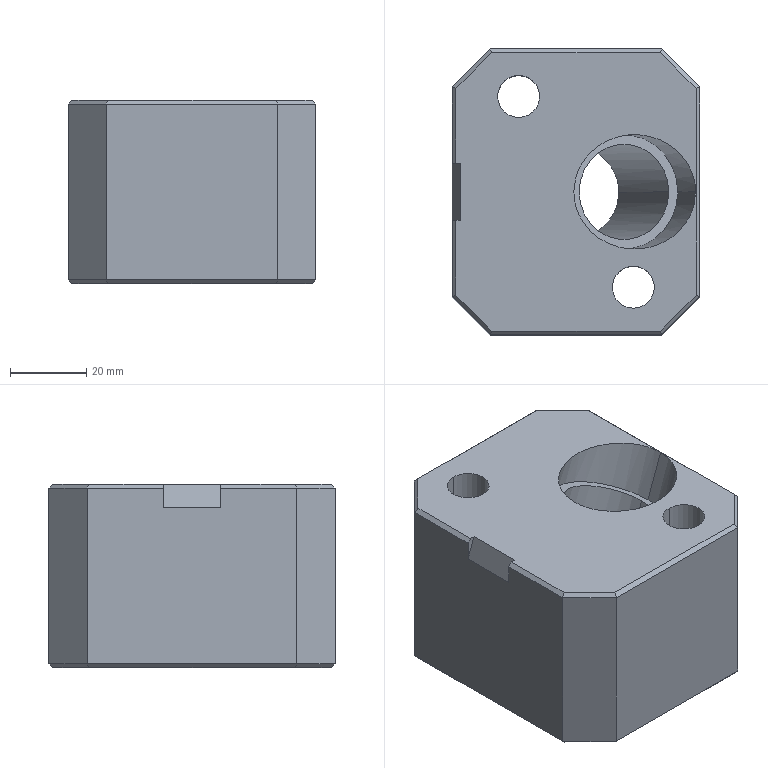Part | Creo | 3 solids | 49 faces | box 65 x 75 x 48 mm | volume 184573 mm3 | plane 33 | cylinder 16 | commonest cylinder face diameters 11 x4 18 x4 11.98 x2 12 x2 25 x2 30 x2
STEP:
#1=CARTESIAN_POINT('',(-250.936,145.997,1.));
#2=VERTEX_POINT('',#1);
#3=CARTESIAN_POINT('',(-250.936,163.997,1.));
#4=VERTEX_POINT('',#3);
#5=CARTESIAN_POINT('',(-250.936,154.997,1.));
#6=DIRECTION('',(0.,0.,-1.));
#7=DIRECTION('',(0.,-1.,0.));
#8=AXIS2_PLACEMENT_3D('',#5,#6,#7);
#9=CIRCLE('',#8,9.);
#10=EDGE_CURVE('',#2,#4,#9,.T.);
#11=ORIENTED_EDGE('',*,*,#10,.F.);
#12=CARTESIAN_POINT('',(-250.936,154.997,1.));
#13=DIRECTION('',(0.,0.,-1.));
#14=DIRECTION('',(0.,1.,0.));
#15=AXIS2_PLACEMENT_3D('',#12,#13,#14);
#16=CIRCLE('',#15,9.);
#17=EDGE_CURVE('',#4,#2,#16,.T.);
#18=ORIENTED_EDGE('',*,*,#17,.F.);
#19=EDGE_LOOP('',(#11,#18));
#20=FACE_OUTER_BOUND('',#19,.F.);
#21=CARTESIAN_POINT('',(-250.936,149.497,1.));
#22=VERTEX_POINT('',#21);
#23=CARTESIAN_POINT('',(-250.936,160.497,1.));
#24=VERTEX_POINT('',#23);
#25=CARTESIAN_POINT('',(-250.936,154.997,1.));
#26=DIRECTION('',(0.,0.,1.));
#27=DIRECTION('',(0.,-1.,0.));
#28=AXIS2_PLACEMENT_3D('',#25,#26,#27);
#29=CIRCLE('',#28,5.5);
#30=EDGE_CURVE('',#22,#24,#29,.T.);
#31=ORIENTED_EDGE('',*,*,#30,.F.);
#32=CARTESIAN_POINT('',(-250.936,154.997,1.));
#33=DIRECTION('',(0.,0.,1.));
#34=DIRECTION('',(0.,1.,0.));
#35=AXIS2_PLACEMENT_3D('',#32,#33,#34);
#36=CIRCLE('',#35,5.5);
#37=EDGE_CURVE('',#24,#22,#36,.T.);
#38=ORIENTED_EDGE('',*,*,#37,.F.);
#39=EDGE_LOOP('',(#31,#38));
#40=FACE_BOUND('',#39,.F.);
#41=CARTESIAN_POINT('',(-250.936,154.997,1.));
#42=DIRECTION('',(0.,0.,1.));
#43=DIRECTION('',(0.,-1.,0.));
#44=AXIS2_PLACEMENT_3D('',#41,#42,#43);
#45=PLANE('',#44);
#46=ADVANCED_FACE('',(#20,#40),#45,.F.);
#47=ORIENTED_EDGE('',*,*,#10,.T.);
#48=CARTESIAN_POINT('',(-250.936,163.997,-10.));
#49=VERTEX_POINT('',#48);
#50=CARTESIAN_POINT('',(-250.936,163.997,-10.));
#51=DIRECTION('',(0.,0.,1.));
#52=VECTOR('',#51,11.);
#53=LINE('',#50,#52);
#54=EDGE_CURVE('',#49,#4,#53,.T.);
#55=ORIENTED_EDGE('',*,*,#54,.F.);
#56=CARTESIAN_POINT('',(-250.936,145.997,-10.));
#57=VERTEX_POINT('',#56);
#58=CARTESIAN_POINT('',(-250.936,154.997,-10.));
#59=DIRECTION('',(0.,0.,1.));
#60=DIRECTION('',(0.,1.,0.));
#61=AXIS2_PLACEMENT_3D('',#58,#59,#60);
#62=CIRCLE('',#61,9.);
#63=EDGE_CURVE('',#49,#57,#62,.T.);
#64=ORIENTED_EDGE('',*,*,#63,.T.);
#65=CARTESIAN_POINT('',(-250.936,145.997,-10.));
#66=DIRECTION('',(0.,0.,1.));
#67=VECTOR('',#66,11.);
#68=LINE('',#65,#67);
#69=EDGE_CURVE('',#57,#2,#68,.T.);
#70=ORIENTED_EDGE('',*,*,#69,.T.);
#71=EDGE_LOOP('',(#47,#55,#64,#70));
#72=FACE_OUTER_BOUND('',#71,.F.);
#73=CARTESIAN_POINT('',(-250.936,154.997,-10.));
#74=DIRECTION('',(0.,0.,1.));
#75=DIRECTION('',(0.,-1.,0.));
#76=AXIS2_PLACEMENT_3D('',#73,#74,#75);
#77=CYLINDRICAL_SURFACE('',#76,9.);
#78=ADVANCED_FACE('',(#72),#77,.F.);
#79=ORIENTED_EDGE('',*,*,#17,.T.);
#80=ORIENTED_EDGE('',*,*,#69,.F.);
#81=CARTESIAN_POINT('',(-250.936,154.997,-10.));
#82=DIRECTION('',(0.,0.,1.));
#83=DIRECTION('',(0.,-1.,0.));
#84=AXIS2_PLACEMENT_3D('',#81,#82,#83);
#85=CIRCLE('',#84,9.);
#86=EDGE_CURVE('',#57,#49,#85,.T.);
#87=ORIENTED_EDGE('',*,*,#86,.T.);
#88=ORIENTED_EDGE('',*,*,#54,.T.);
#89=EDGE_LOOP('',(#79,#80,#87,#88));
#90=FACE_OUTER_BOUND('',#89,.F.);
#91=CARTESIAN_POINT('',(-250.936,154.997,-10.));
#92=DIRECTION('',(0.,0.,1.));
#93=DIRECTION('',(0.,-1.,0.));
#94=AXIS2_PLACEMENT_3D('',#91,#92,#93);
#95=CYLINDRICAL_SURFACE('',#94,9.);
#96=ADVANCED_FACE('',(#90),#95,.F.);
#97=CARTESIAN_POINT('',(-213.85,166.497,-10.));
#98=VERTEX_POINT('',#97);
#99=CARTESIAN_POINT('',(-204.436,157.083,-10.));
#100=VERTEX_POINT('',#99);
#101=CARTESIAN_POINT('',(-213.85,166.497,-10.));
#102=DIRECTION('',(0.7071,-0.7071,0.));
#103=VECTOR('',#102,13.314);
#104=LINE('',#101,#103);
#105=EDGE_CURVE('',#98,#100,#104,.T.);
#106=ORIENTED_EDGE('',*,*,#105,.F.);
#107=CARTESIAN_POINT('',(-258.022,166.497,-10.));
#108=VERTEX_POINT('',#107);
#109=CARTESIAN_POINT('',(-213.85,166.497,-10.));
#110=DIRECTION('',(-1.,0.,0.));
#111=VECTOR('',#110,44.172);
#112=LINE('',#109,#111);
#113=EDGE_CURVE('',#98,#108,#112,.T.);
#114=ORIENTED_EDGE('',*,*,#113,.T.);
#115=CARTESIAN_POINT('',(-267.436,157.083,-10.));
#116=VERTEX_POINT('',#115);
#117=CARTESIAN_POINT('',(-267.436,157.083,-10.));
#118=DIRECTION('',(0.7071,0.7071,0.));
#119=VECTOR('',#118,13.314);
#120=LINE('',#117,#119);
#121=EDGE_CURVE('',#116,#108,#120,.T.);
#122=ORIENTED_EDGE('',*,*,#121,.F.);
#123=CARTESIAN_POINT('',(-267.436,102.911,-10.));
#124=VERTEX_POINT('',#123);
#125=CARTESIAN_POINT('',(-267.436,157.083,-10.));
#126=DIRECTION('',(0.,-1.,0.));
#127=VECTOR('',#126,54.172);
#128=LINE('',#125,#127);
#129=EDGE_CURVE('',#116,#124,#128,.T.);
#130=ORIENTED_EDGE('',*,*,#129,.T.);
#131=CARTESIAN_POINT('',(-258.022,93.497,-10.));
#132=VERTEX_POINT('',#131);
#133=CARTESIAN_POINT('',(-258.022,93.497,-10.));
#134=DIRECTION('',(-0.7071,0.7071,0.));
#135=VECTOR('',#134,13.314);
#136=LINE('',#133,#135);
#137=EDGE_CURVE('',#132,#124,#136,.T.);
#138=ORIENTED_EDGE('',*,*,#137,.F.);
#139=CARTESIAN_POINT('',(-213.85,93.497,-10.));
#140=VERTEX_POINT('',#139);
#141=CARTESIAN_POINT('',(-258.022,93.497,-10.));
#142=DIRECTION('',(1.,0.,0.));
#143=VECTOR('',#142,44.172);
#144=LINE('',#141,#143);
#145=EDGE_CURVE('',#132,#140,#144,.T.);
#146=ORIENTED_EDGE('',*,*,#145,.T.);
#147=CARTESIAN_POINT('',(-204.436,102.911,-10.));
#148=VERTEX_POINT('',#147);
#149=CARTESIAN_POINT('',(-204.436,102.911,-10.));
#150=DIRECTION('',(-0.7071,-0.7071,0.));
#151=VECTOR('',#150,13.314);
#152=LINE('',#149,#151);
#153=EDGE_CURVE('',#148,#140,#152,.T.);
#154=ORIENTED_EDGE('',*,*,#153,.F.);
#155=CARTESIAN_POINT('',(-204.436,102.911,-10.));
#156=DIRECTION('',(0.,1.,0.));
#157=VECTOR('',#156,54.172);
#158=LINE('',#155,#157);
#159=EDGE_CURVE('',#148,#100,#158,.T.);
#160=ORIENTED_EDGE('',*,*,#159,.T.);
#161=EDGE_LOOP('',(#106,#114,#122,#130,#138,#146,#154,#160));
#162=FACE_OUTER_BOUND('',#161,.F.);
#163=CARTESIAN_POINT('',(-224.707,129.995,-10.));
#164=VERTEX_POINT('',#163);
#165=CARTESIAN_POINT('',(-251.311,129.995,-10.));
#166=VERTEX_POINT('',#165);
#167=CARTESIAN_POINT('',(-224.707,129.995,-10.));
#168=CARTESIAN_POINT('',(-224.707,128.522,-10.));
#169=CARTESIAN_POINT('',(-225.275,125.338,-10.));
#170=CARTESIAN_POINT('',(-227.815,121.638,-10.));
#171=CARTESIAN_POINT('',(-230.687,119.454,-10.));
#172=CARTESIAN_POINT('',(-233.098,118.289,-10.));
#173=CARTESIAN_POINT('',(-235.181,117.737,-10.));
#174=CARTESIAN_POINT('',(-236.821,117.528,-10.));
#175=CARTESIAN_POINT('',(-238.009,117.479,-10.));
#176=CARTESIAN_POINT('',(-239.198,117.528,-10.));
#177=CARTESIAN_POINT('',(-240.838,117.737,-10.));
#178=CARTESIAN_POINT('',(-242.921,118.289,-10.));
#179=CARTESIAN_POINT('',(-245.331,119.454,-10.));
#180=CARTESIAN_POINT('',(-248.203,121.638,-10.));
#181=CARTESIAN_POINT('',(-250.743,125.338,-10.));
#182=CARTESIAN_POINT('',(-251.311,128.522,-10.));
#183=CARTESIAN_POINT('',(-251.311,129.995,-10.));
#184=B_SPLINE_CURVE_WITH_KNOTS('',3,(#167,#168,#169,#170,#171,#172,#173,#174,#175,#176,#177,#178,#179,#180,#181,#182,#183),.UNSPECIFIED.,.F.,.F.,(4,1,1,1,1,1,1,1,1,1,1,1,1,1,4),(0.,0.125,0.25,0.3125,0.375,0.4375,0.4688,0.5,0.5312,0.5625,0.625,0.6875,0.75,0.875,1.),.UNSPECIFIED.);
#185=EDGE_CURVE('',#164,#166,#184,.T.);
#186=ORIENTED_EDGE('',*,*,#185,.T.);
#187=CARTESIAN_POINT('',(-251.311,129.995,-10.));
#188=CARTESIAN_POINT('',(-251.311,131.468,-10.));
#189=CARTESIAN_POINT('',(-250.743,134.652,-10.));
#190=CARTESIAN_POINT('',(-248.203,138.353,-10.));
#191=CARTESIAN_POINT('',(-245.331,140.537,-10.));
#192=CARTESIAN_POINT('',(-242.921,141.701,-10.));
#193=CARTESIAN_POINT('',(-240.838,142.254,-10.));
#194=CARTESIAN_POINT('',(-239.198,142.463,-10.));
#195=CARTESIAN_POINT('',(-238.009,142.512,-10.));
#196=CARTESIAN_POINT('',(-236.821,142.463,-10.));
#197=CARTESIAN_POINT('',(-235.181,142.254,-10.));
#198=CARTESIAN_POINT('',(-233.098,141.701,-10.));
#199=CARTESIAN_POINT('',(-230.687,140.537,-10.));
#200=CARTESIAN_POINT('',(-227.815,138.353,-10.));
#201=CARTESIAN_POINT('',(-225.275,134.652,-10.));
#202=CARTESIAN_POINT('',(-224.707,131.468,-10.));
#203=CARTESIAN_POINT('',(-224.707,129.995,-10.));
#204=B_SPLINE_CURVE_WITH_KNOTS('',3,(#187,#188,#189,#190,#191,#192,#193,#194,#195,#196,#197,#198,#199,#200,#201,#202,#203),.UNSPECIFIED.,.F.,.F.,(4,1,1,1,1,1,1,1,1,1,1,1,1,1,4),(0.,0.125,0.25,0.3125,0.375,0.4375,0.4688,0.5,0.5312,0.5625,0.625,0.6875,0.75,0.875,1.),.UNSPECIFIED.);
#205=EDGE_CURVE('',#166,#164,#204,.T.);
#206=ORIENTED_EDGE('',*,*,#205,.T.);
#207=EDGE_LOOP('',(#186,#206));
#208=FACE_BOUND('',#207,.F.);
#209=ORIENTED_EDGE('',*,*,#86,.F.);
#210=ORIENTED_EDGE('',*,*,#63,.F.);
#211=EDGE_LOOP('',(#209,#210));
#212=FACE_BOUND('',#211,.F.);
#213=CARTESIAN_POINT('',(-220.936,95.997,-10.));
#214=VERTEX_POINT('',#213);
#215=CARTESIAN_POINT('',(-220.936,113.997,-10.));
#216=VERTEX_POINT('',#215);
#217=CARTESIAN_POINT('',(-220.936,104.997,-10.));
#218=DIRECTION('',(0.,0.,1.));
#219=DIRECTION('',(0.,-1.,0.));
#220=AXIS2_PLACEMENT_3D('',#217,#218,#219);
#221=CIRCLE('',#220,9.);
#222=EDGE_CURVE('',#214,#216,#221,.T.);
#223=ORIENTED_EDGE('',*,*,#222,.F.);
#224=CARTESIAN_POINT('',(-220.936,104.997,-10.));
#225=DIRECTION('',(0.,0.,1.));
#226=DIRECTION('',(0.,1.,0.));
#227=AXIS2_PLACEMENT_3D('',#224,#225,#226);
#228=CIRCLE('',#227,9.);
#229=EDGE_CURVE('',#216,#214,#228,.T.);
#230=ORIENTED_EDGE('',*,*,#229,.F.);
#231=EDGE_LOOP('',(#223,#230));
#232=FACE_BOUND('',#231,.F.);
#233=CARTESIAN_POINT('',(605.564,160.997,-10.));
#234=DIRECTION('',(0.,0.,1.));
#235=DIRECTION('',(-1.,0.,0.));
#236=AXIS2_PLACEMENT_3D('',#233,#234,#235);
#237=PLANE('',#236);
#238=ADVANCED_FACE('',(#162,#208,#212,#232),#237,.F.);
#239=CARTESIAN_POINT('',(-211.613,129.995,25.977));
#240=VERTEX_POINT('',#239);
#241=CARTESIAN_POINT('',(-235.105,129.995,34.527));
#242=VERTEX_POINT('',#241);
#243=CARTESIAN_POINT('',(-223.359,129.995,30.252));
#244=DIRECTION('',(-0.342,0.,-0.9397));
#245=DIRECTION('',(0.9397,0.,-0.342));
#246=AXIS2_PLACEMENT_3D('',#243,#244,#245);
#247=CIRCLE('',#246,12.5);
#248=EDGE_CURVE('',#240,#242,#247,.T.);
#249=ORIENTED_EDGE('',*,*,#248,.T.);
#250=CARTESIAN_POINT('',(-235.105,129.995,34.527));
#251=DIRECTION('',(-0.342,0.,-0.9397));
#252=VECTOR('',#251,47.385);
#253=LINE('',#250,#252);
#254=EDGE_CURVE('',#242,#166,#253,.T.);
#255=ORIENTED_EDGE('',*,*,#254,.T.);
#256=ORIENTED_EDGE('',*,*,#185,.F.);
#257=CARTESIAN_POINT('',(-211.613,129.995,25.977));
#258=DIRECTION('',(-0.342,0.,-0.9397));
#259=VECTOR('',#258,38.286);
#260=LINE('',#257,#259);
#261=EDGE_CURVE('',#240,#164,#260,.T.);
#262=ORIENTED_EDGE('',*,*,#261,.F.);
#263=EDGE_LOOP('',(#249,#255,#256,#262));
#264=FACE_OUTER_BOUND('',#263,.F.);
#265=CARTESIAN_POINT('',(-211.802,129.995,62.004));
#266=DIRECTION('',(-0.342,0.,-0.9397));
#267=DIRECTION('',(-0.9397,0.,0.342));
#268=AXIS2_PLACEMENT_3D('',#265,#266,#267);
#269=CYLINDRICAL_SURFACE('',#268,12.5);
#270=ADVANCED_FACE('',(#264),#269,.F.);
#271=CARTESIAN_POINT('',(-209.263,129.995,25.122));
#272=VERTEX_POINT('',#271);
#273=CARTESIAN_POINT('',(-237.454,129.995,35.382));
#274=VERTEX_POINT('',#273);
#275=CARTESIAN_POINT('',(-223.359,129.995,30.252));
#276=DIRECTION('',(0.342,0.,0.9397));
#277=DIRECTION('',(0.9397,0.,-0.342));
#278=AXIS2_PLACEMENT_3D('',#275,#276,#277);
#279=CIRCLE('',#278,15.);
#280=EDGE_CURVE('',#272,#274,#279,.T.);
#281=ORIENTED_EDGE('',*,*,#280,.F.);
#282=CARTESIAN_POINT('',(-223.359,129.995,30.252));
#283=DIRECTION('',(0.342,0.,0.9397));
#284=DIRECTION('',(-0.9397,0.,0.342));
#285=AXIS2_PLACEMENT_3D('',#282,#283,#284);
#286=CIRCLE('',#285,15.);
#287=EDGE_CURVE('',#274,#272,#286,.T.);
#288=ORIENTED_EDGE('',*,*,#287,.F.);
#289=EDGE_LOOP('',(#281,#288));
#290=FACE_OUTER_BOUND('',#289,.F.);
#291=ORIENTED_EDGE('',*,*,#248,.F.);
#292=CARTESIAN_POINT('',(-223.359,129.995,30.252));
#293=DIRECTION('',(-0.342,0.,-0.9397));
#294=DIRECTION('',(-0.9397,0.,0.342));
#295=AXIS2_PLACEMENT_3D('',#292,#293,#294);
#296=CIRCLE('',#295,12.5);
#297=EDGE_CURVE('',#242,#240,#296,.T.);
#298=ORIENTED_EDGE('',*,*,#297,.F.);
#299=EDGE_LOOP('',(#291,#298));
#300=FACE_BOUND('',#299,.F.);
#301=CARTESIAN_POINT('',(-223.359,129.995,30.252));
#302=DIRECTION('',(-0.342,0.,-0.9397));
#303=DIRECTION('',(-0.9397,0.,0.342));
#304=AXIS2_PLACEMENT_3D('',#301,#302,#303);
#305=PLANE('',#304);
#306=ADVANCED_FACE('',(#290,#300),#305,.F.);
#307=ORIENTED_EDGE('',*,*,#297,.T.);
#308=ORIENTED_EDGE('',*,*,#261,.T.);
#309=ORIENTED_EDGE('',*,*,#205,.F.);
#310=ORIENTED_EDGE('',*,*,#254,.F.);
#311=EDGE_LOOP('',(#307,#308,#309,#310));
#312=FACE_OUTER_BOUND('',#311,.F.);
#313=CARTESIAN_POINT('',(-211.802,129.995,62.004));
#314=DIRECTION('',(-0.342,0.,-0.9397));
#315=DIRECTION('',(-0.9397,0.,0.342));
#316=AXIS2_PLACEMENT_3D('',#313,#314,#315);
#317=CYLINDRICAL_SURFACE('',#316,12.5);
#318=ADVANCED_FACE('',(#312),#317,.F.);
#319=CARTESIAN_POINT('',(-236.501,129.995,38.));
#320=VERTEX_POINT('',#319);
#321=CARTESIAN_POINT('',(-204.576,129.995,38.));
#322=VERTEX_POINT('',#321);
#323=CARTESIAN_POINT('',(-236.501,129.995,38.));
#324=CARTESIAN_POINT('',(-236.501,131.763,38.));
#325=CARTESIAN_POINT('',(-235.82,135.584,38.));
#326=CARTESIAN_POINT('',(-232.772,140.025,38.));
#327=CARTESIAN_POINT('',(-229.325,142.645,38.));
#328=CARTESIAN_POINT('',(-226.432,144.042,38.));
#329=CARTESIAN_POINT('',(-223.933,144.706,38.));
#330=CARTESIAN_POINT('',(-221.965,144.956,38.));
#331=CARTESIAN_POINT('',(-220.539,145.015,38.));
#332=CARTESIAN_POINT('',(-219.113,144.956,38.));
#333=CARTESIAN_POINT('',(-217.145,144.706,38.));
#334=CARTESIAN_POINT('',(-214.645,144.042,38.));
#335=CARTESIAN_POINT('',(-211.752,142.645,38.));
#336=CARTESIAN_POINT('',(-208.306,140.025,38.));
#337=CARTESIAN_POINT('',(-205.258,135.584,38.));
#338=CARTESIAN_POINT('',(-204.576,131.763,38.));
#339=CARTESIAN_POINT('',(-204.576,129.995,38.));
#340=B_SPLINE_CURVE_WITH_KNOTS('',3,(#323,#324,#325,#326,#327,#328,#329,#330,#331,#332,#333,#334,#335,#336,#337,#338,#339),.UNSPECIFIED.,.F.,.F.,(4,1,1,1,1,1,1,1,1,1,1,1,1,1,4),(0.,0.125,0.25,0.3125,0.375,0.4375,0.4688,0.5,0.5312,0.5625,0.625,0.6875,0.75,0.875,1.),.UNSPECIFIED.);
#341=EDGE_CURVE('',#320,#322,#340,.T.);
#342=ORIENTED_EDGE('',*,*,#341,.T.);
#343=CARTESIAN_POINT('',(-204.576,129.995,38.));
#344=DIRECTION('',(-0.342,0.,-0.9397));
#345=VECTOR('',#344,13.705);
#346=LINE('',#343,#345);
#347=EDGE_CURVE('',#322,#272,#346,.T.);
#348=ORIENTED_EDGE('',*,*,#347,.T.);
#349=ORIENTED_EDGE('',*,*,#280,.T.);
#350=CARTESIAN_POINT('',(-236.501,129.995,38.));
#351=DIRECTION('',(-0.342,0.,-0.9397));
#352=VECTOR('',#351,2.786);
#353=LINE('',#350,#352);
#354=EDGE_CURVE('',#320,#274,#353,.T.);
#355=ORIENTED_EDGE('',*,*,#354,.F.);
#356=EDGE_LOOP('',(#342,#348,#349,#355));
#357=FACE_OUTER_BOUND('',#356,.F.);
#358=CARTESIAN_POINT('',(-217.527,129.995,46.274));
#359=DIRECTION('',(-0.342,0.,-0.9397));
#360=DIRECTION('',(-0.9397,0.,0.342));
#361=AXIS2_PLACEMENT_3D('',#358,#359,#360);
#362=CYLINDRICAL_SURFACE('',#361,15.);
#363=ADVANCED_FACE('',(#357),#362,.F.);
#364=CARTESIAN_POINT('',(-266.228,122.497,38.));
#365=VERTEX_POINT('',#364);
#366=CARTESIAN_POINT('',(-267.436,122.497,38.));
#367=VERTEX_POINT('',#366);
#368=CARTESIAN_POINT('',(-266.228,122.497,38.));
#369=DIRECTION('',(-1.,0.,0.));
#370=VECTOR('',#369,1.208);
#371=LINE('',#368,#370);
#372=EDGE_CURVE('',#365,#367,#371,.T.);
#373=ORIENTED_EDGE('',*,*,#372,.F.);
#374=CARTESIAN_POINT('',(-266.228,137.497,38.));
#375=VERTEX_POINT('',#374);
#376=CARTESIAN_POINT('',(-266.228,137.497,38.));
#377=DIRECTION('',(0.,-1.,0.));
#378=VECTOR('',#377,15.);
#379=LINE('',#376,#378);
#380=EDGE_CURVE('',#375,#365,#379,.T.);
#381=ORIENTED_EDGE('',*,*,#380,.F.);
#382=CARTESIAN_POINT('',(-267.436,137.497,38.));
#383=VERTEX_POINT('',#382);
#384=CARTESIAN_POINT('',(-267.436,137.497,38.));
#385=DIRECTION('',(1.,0.,0.));
#386=VECTOR('',#385,1.208);
#387=LINE('',#384,#386);
#388=EDGE_CURVE('',#383,#375,#387,.T.);
#389=ORIENTED_EDGE('',*,*,#388,.F.);
#390=CARTESIAN_POINT('',(-267.436,157.083,38.));
#391=VERTEX_POINT('',#390);
#392=CARTESIAN_POINT('',(-267.436,137.497,38.));
#393=DIRECTION('',(0.,1.,0.));
#394=VECTOR('',#393,19.586);
#395=LINE('',#392,#394);
#396=EDGE_CURVE('',#383,#391,#395,.T.);
#397=ORIENTED_EDGE('',*,*,#396,.T.);
#398=CARTESIAN_POINT('',(-258.022,166.497,38.));
#399=VERTEX_POINT('',#398);
#400=CARTESIAN_POINT('',(-258.022,166.497,38.));
#401=DIRECTION('',(-0.7071,-0.7071,0.));
#402=VECTOR('',#401,13.314);
#403=LINE('',#400,#402);
#404=EDGE_CURVE('',#399,#391,#403,.T.);
#405=ORIENTED_EDGE('',*,*,#404,.F.);
#406=CARTESIAN_POINT('',(-213.85,166.497,38.));
#407=VERTEX_POINT('',#406);
#408=CARTESIAN_POINT('',(-258.022,166.497,38.));
#409=DIRECTION('',(1.,0.,0.));
#410=VECTOR('',#409,44.172);
#411=LINE('',#408,#410);
#412=EDGE_CURVE('',#399,#407,#411,.T.);
#413=ORIENTED_EDGE('',*,*,#412,.T.);
#414=CARTESIAN_POINT('',(-204.436,157.083,38.));
#415=VERTEX_POINT('',#414);
#416=CARTESIAN_POINT('',(-204.436,157.083,38.));
#417=DIRECTION('',(-0.7071,0.7071,0.));
#418=VECTOR('',#417,13.314);
#419=LINE('',#416,#418);
#420=EDGE_CURVE('',#415,#407,#419,.T.);
#421=ORIENTED_EDGE('',*,*,#420,.F.);
#422=CARTESIAN_POINT('',(-204.436,102.911,38.));
#423=VERTEX_POINT('',#422);
#424=CARTESIAN_POINT('',(-204.436,157.083,38.));
#425=DIRECTION('',(0.,-1.,0.));
#426=VECTOR('',#425,54.172);
#427=LINE('',#424,#426);
#428=EDGE_CURVE('',#415,#423,#427,.T.);
#429=ORIENTED_EDGE('',*,*,#428,.T.);
#430=CARTESIAN_POINT('',(-213.85,93.497,38.));
#431=VERTEX_POINT('',#430);
#432=CARTESIAN_POINT('',(-213.85,93.497,38.));
#433=DIRECTION('',(0.7071,0.7071,0.));
#434=VECTOR('',#433,13.314);
#435=LINE('',#432,#434);
#436=EDGE_CURVE('',#431,#423,#435,.T.);
#437=ORIENTED_EDGE('',*,*,#436,.F.);
#438=CARTESIAN_POINT('',(-258.022,93.497,38.));
#439=VERTEX_POINT('',#438);
#440=CARTESIAN_POINT('',(-213.85,93.497,38.));
#441=DIRECTION('',(-1.,0.,0.));
#442=VECTOR('',#441,44.172);
#443=LINE('',#440,#442);
#444=EDGE_CURVE('',#431,#439,#443,.T.);
#445=ORIENTED_EDGE('',*,*,#444,.T.);
#446=CARTESIAN_POINT('',(-267.436,102.911,38.));
#447=VERTEX_POINT('',#446);
#448=CARTESIAN_POINT('',(-267.436,102.911,38.));
#449=DIRECTION('',(0.7071,-0.7071,0.));
#450=VECTOR('',#449,13.314);
#451=LINE('',#448,#450);
#452=EDGE_CURVE('',#447,#439,#451,.T.);
#453=ORIENTED_EDGE('',*,*,#452,.F.);
#454=CARTESIAN_POINT('',(-267.436,102.911,38.));
#455=DIRECTION('',(0.,1.,0.));
#456=VECTOR('',#455,19.586);
#457=LINE('',#454,#456);
#458=EDGE_CURVE('',#447,#367,#457,.T.);
#459=ORIENTED_EDGE('',*,*,#458,.T.);
#460=EDGE_LOOP('',(#373,#381,#389,#397,#405,#413,#421,#429,#437,#445,#453,#459));
#461=FACE_OUTER_BOUND('',#460,.F.);
#462=CARTESIAN_POINT('',(-250.936,149.497,38.));
#463=VERTEX_POINT('',#462);
#464=CARTESIAN_POINT('',(-250.936,160.497,38.));
#465=VERTEX_POINT('',#464);
#466=CARTESIAN_POINT('',(-250.936,154.997,38.));
#467=DIRECTION('',(0.,0.,-1.));
#468=DIRECTION('',(0.,-1.,0.));
#469=AXIS2_PLACEMENT_3D('',#466,#467,#468);
#470=CIRCLE('',#469,5.5);
#471=EDGE_CURVE('',#463,#465,#470,.T.);
#472=ORIENTED_EDGE('',*,*,#471,.F.);
#473=CARTESIAN_POINT('',(-250.936,154.997,38.));
#474=DIRECTION('',(0.,0.,-1.));
#475=DIRECTION('',(0.,1.,0.));
#476=AXIS2_PLACEMENT_3D('',#473,#474,#475);
#477=CIRCLE('',#476,5.5);
#478=EDGE_CURVE('',#465,#463,#477,.T.);
#479=ORIENTED_EDGE('',*,*,#478,.F.);
#480=EDGE_LOOP('',(#472,#479));
#481=FACE_BOUND('',#480,.F.);
#482=CARTESIAN_POINT('',(-220.936,99.497,38.));
#483=VERTEX_POINT('',#482);
#484=CARTESIAN_POINT('',(-220.936,110.497,38.));
#485=VERTEX_POINT('',#484);
#486=CARTESIAN_POINT('',(-220.936,104.997,38.));
#487=DIRECTION('',(0.,0.,-1.));
#488=DIRECTION('',(0.,-1.,0.));
#489=AXIS2_PLACEMENT_3D('',#486,#487,#488);
#490=CIRCLE('',#489,5.5);
#491=EDGE_CURVE('',#483,#485,#490,.T.);
#492=ORIENTED_EDGE('',*,*,#491,.F.);
#493=CARTESIAN_POINT('',(-220.936,104.997,38.));
#494=DIRECTION('',(0.,0.,-1.));
#495=DIRECTION('',(0.,1.,0.));
#496=AXIS2_PLACEMENT_3D('',#493,#494,#495);
#497=CIRCLE('',#496,5.5);
#498=EDGE_CURVE('',#485,#483,#497,.T.);
#499=ORIENTED_EDGE('',*,*,#498,.F.);
#500=EDGE_LOOP('',(#492,#499));
#501=FACE_BOUND('',#500,.F.);
#502=ORIENTED_EDGE('',*,*,#341,.F.);
#503=CARTESIAN_POINT('',(-204.576,129.995,38.));
#504=CARTESIAN_POINT('',(-204.576,128.228,38.));
#505=CARTESIAN_POINT('',(-205.258,124.407,38.));
#506=CARTESIAN_POINT('',(-208.306,119.966,38.));
#507=CARTESIAN_POINT('',(-211.752,117.346,38.));
#508=CARTESIAN_POINT('',(-214.645,115.948,38.));
#509=CARTESIAN_POINT('',(-217.145,115.285,38.));
#510=CARTESIAN_POINT('',(-219.113,115.034,38.));
#511=CARTESIAN_POINT('',(-220.539,114.976,38.));
#512=CARTESIAN_POINT('',(-221.965,115.034,38.));
#513=CARTESIAN_POINT('',(-223.933,115.285,38.));
#514=CARTESIAN_POINT('',(-226.432,115.948,38.));
#515=CARTESIAN_POINT('',(-229.325,117.346,38.));
#516=CARTESIAN_POINT('',(-232.772,119.966,38.));
#517=CARTESIAN_POINT('',(-235.82,124.407,38.));
#518=CARTESIAN_POINT('',(-236.501,128.228,38.));
#519=CARTESIAN_POINT('',(-236.501,129.995,38.));
#520=B_SPLINE_CURVE_WITH_KNOTS('',3,(#503,#504,#505,#506,#507,#508,#509,#510,#511,#512,#513,#514,#515,#516,#517,#518,#519),.UNSPECIFIED.,.F.,.F.,(4,1,1,1,1,1,1,1,1,1,1,1,1,1,4),(0.,0.125,0.25,0.3125,0.375,0.4375,0.4688,0.5,0.5312,0.5625,0.625,0.6875,0.75,0.875,1.),.UNSPECIFIED.);
#521=EDGE_CURVE('',#322,#320,#520,.T.);
#522=ORIENTED_EDGE('',*,*,#521,.F.);
#523=EDGE_LOOP('',(#502,#522));
#524=FACE_BOUND('',#523,.F.);
#525=CARTESIAN_POINT('',(-222.833,-235.939,38.));
#526=DIRECTION('',(0.,0.,1.));
#527=DIRECTION('',(0.,1.,0.));
#528=AXIS2_PLACEMENT_3D('',#525,#526,#527);
#529=PLANE('',#528);
#530=ADVANCED_FACE('',(#461,#481,#501,#524),#529,.T.);
#531=ORIENTED_EDGE('',*,*,#372,.T.);
#532=CARTESIAN_POINT('',(-268.436,122.497,37.));
#533=VERTEX_POINT('',#532);
#534=CARTESIAN_POINT('',(-268.436,122.497,37.));
#535=DIRECTION('',(0.7071,0.,0.7071));
#536=VECTOR('',#535,1.414);
#537=LINE('',#534,#536);
#538=EDGE_CURVE('',#533,#367,#537,.T.);
#539=ORIENTED_EDGE('',*,*,#538,.F.);
#540=CARTESIAN_POINT('',(-268.436,122.497,31.933));
#541=VERTEX_POINT('',#540);
#542=CARTESIAN_POINT('',(-268.436,122.497,37.));
#543=DIRECTION('',(0.,0.,-1.));
#544=VECTOR('',#543,5.067);
#545=LINE('',#542,#544);
#546=EDGE_CURVE('',#533,#541,#545,.T.);
#547=ORIENTED_EDGE('',*,*,#546,.T.);
#548=CARTESIAN_POINT('',(-266.228,122.497,38.));
#549=DIRECTION('',(-0.342,0.,-0.9397));
#550=VECTOR('',#549,6.456);
#551=LINE('',#548,#550);
#552=EDGE_CURVE('',#365,#541,#551,.T.);
#553=ORIENTED_EDGE('',*,*,#552,.F.);
#554=EDGE_LOOP('',(#531,#539,#547,#553));
#555=FACE_OUTER_BOUND('',#554,.F.);
#556=CARTESIAN_POINT('',(-289.218,122.497,-1.436));
#557=DIRECTION('',(0.,-1.,0.));
#558=DIRECTION('',(0.,0.,-1.));
#559=AXIS2_PLACEMENT_3D('',#556,#557,#558);
#560=PLANE('',#559);
#561=ADVANCED_FACE('',(#555),#560,.F.);
#562=ORIENTED_EDGE('',*,*,#538,.T.);
#563=ORIENTED_EDGE('',*,*,#458,.F.);
#564=CARTESIAN_POINT('',(-268.436,102.497,37.));
#565=VERTEX_POINT('',#564);
#566=CARTESIAN_POINT('',(-268.436,102.497,37.));
#567=DIRECTION('',(0.6786,0.2811,0.6786));
#568=VECTOR('',#567,1.474);
#569=LINE('',#566,#568);
#570=EDGE_CURVE('',#565,#447,#569,.T.);
#571=ORIENTED_EDGE('',*,*,#570,.F.);
#572=CARTESIAN_POINT('',(-268.436,122.497,37.));
#573=DIRECTION('',(0.,-1.,0.));
#574=VECTOR('',#573,20.);
#575=LINE('',#572,#574);
#576=EDGE_CURVE('',#533,#565,#575,.T.);
#577=ORIENTED_EDGE('',*,*,#576,.F.);
#578=EDGE_LOOP('',(#562,#563,#571,#577));
#579=FACE_OUTER_BOUND('',#578,.F.);
#580=CARTESIAN_POINT('',(-267.436,-235.939,38.));
#581=DIRECTION('',(0.7071,0.,-0.7071));
#582=DIRECTION('',(0.,-1.,0.));
#583=AXIS2_PLACEMENT_3D('',#580,#581,#582);
#584=PLANE('',#583);
#585=ADVANCED_FACE('',(#579),#584,.F.);
#586=ORIENTED_EDGE('',*,*,#452,.T.);
#587=CARTESIAN_POINT('',(-258.436,92.497,37.));
#588=VERTEX_POINT('',#587);
#589=CARTESIAN_POINT('',(-258.436,92.497,37.));
#590=DIRECTION('',(0.2811,0.6786,0.6786));
#591=VECTOR('',#590,1.474);
#592=LINE('',#589,#591);
#593=EDGE_CURVE('',#588,#439,#592,.T.);
#594=ORIENTED_EDGE('',*,*,#593,.F.);
#595=CARTESIAN_POINT('',(-268.436,102.497,37.));
#596=DIRECTION('',(0.7071,-0.7071,0.));
#597=VECTOR('',#596,14.142);
#598=LINE('',#595,#597);
#599=EDGE_CURVE('',#565,#588,#598,.T.);
#600=ORIENTED_EDGE('',*,*,#599,.F.);
#601=ORIENTED_EDGE('',*,*,#570,.T.);
#602=EDGE_LOOP('',(#586,#594,#600,#601));
#603=FACE_OUTER_BOUND('',#602,.F.);
#604=CARTESIAN_POINT('',(-75.709,-88.815,38.));
#605=DIRECTION('',(0.5,0.5,-0.7071));
#606=DIRECTION('',(0.7071,-0.7071,0.));
#607=AXIS2_PLACEMENT_3D('',#604,#605,#606);
#608=PLANE('',#607);
#609=ADVANCED_FACE('',(#603),#608,.F.);
#610=ORIENTED_EDGE('',*,*,#593,.T.);
#611=ORIENTED_EDGE('',*,*,#444,.F.);
#612=CARTESIAN_POINT('',(-213.436,92.497,37.));
#613=VERTEX_POINT('',#612);
#614=CARTESIAN_POINT('',(-213.436,92.497,37.));
#615=DIRECTION('',(-0.2811,0.6786,0.6786));
#616=VECTOR('',#615,1.474);
#617=LINE('',#614,#616);
#618=EDGE_CURVE('',#613,#431,#617,.T.);
#619=ORIENTED_EDGE('',*,*,#618,.F.);
#620=CARTESIAN_POINT('',(-258.436,92.497,37.));
#621=DIRECTION('',(1.,0.,0.));
#622=VECTOR('',#621,45.);
#623=LINE('',#620,#622);
#624=EDGE_CURVE('',#588,#613,#623,.T.);
#625=ORIENTED_EDGE('',*,*,#624,.F.);
#626=EDGE_LOOP('',(#610,#611,#619,#625));
#627=FACE_OUTER_BOUND('',#626,.F.);
#628=CARTESIAN_POINT('',(-222.833,93.497,38.));
#629=DIRECTION('',(0.,-0.7071,0.7071));
#630=DIRECTION('',(-1.,0.,0.));
#631=AXIS2_PLACEMENT_3D('',#628,#629,#630);
#632=PLANE('',#631);
#633=ADVANCED_FACE('',(#627),#632,.T.);
#634=ORIENTED_EDGE('',*,*,#618,.T.);
#635=ORIENTED_EDGE('',*,*,#436,.T.);
#636=CARTESIAN_POINT('',(-203.436,102.497,37.));
#637=VERTEX_POINT('',#636);
#638=CARTESIAN_POINT('',(-203.436,102.497,37.));
#639=DIRECTION('',(-0.6786,0.2811,0.6786));
#640=VECTOR('',#639,1.474);
#641=LINE('',#638,#640);
#642=EDGE_CURVE('',#637,#423,#641,.T.);
#643=ORIENTED_EDGE('',*,*,#642,.F.);
#644=CARTESIAN_POINT('',(-213.436,92.497,37.));
#645=DIRECTION('',(0.7071,0.7071,0.));
#646=VECTOR('',#645,14.142);
#647=LINE('',#644,#646);
#648=EDGE_CURVE('',#613,#637,#647,.T.);
#649=ORIENTED_EDGE('',*,*,#648,.F.);
#650=EDGE_LOOP('',(#634,#635,#643,#649));
#651=FACE_OUTER_BOUND('',#650,.F.);
#652=CARTESIAN_POINT('',(-383.06,-75.713,38.));
#653=DIRECTION('',(-0.5,0.5,-0.7071));
#654=DIRECTION('',(0.7071,0.7071,0.));
#655=AXIS2_PLACEMENT_3D('',#652,#653,#654);
#656=PLANE('',#655);
#657=ADVANCED_FACE('',(#651),#656,.F.);
#658=CARTESIAN_POINT('',(-203.436,157.497,37.));
#659=VERTEX_POINT('',#658);
#660=CARTESIAN_POINT('',(-203.436,157.497,37.));
#661=DIRECTION('',(-0.6786,-0.2811,0.6786));
#662=VECTOR('',#661,1.474);
#663=LINE('',#660,#662);
#664=EDGE_CURVE('',#659,#415,#663,.T.);
#665=ORIENTED_EDGE('',*,*,#664,.F.);
#666=CARTESIAN_POINT('',(-203.436,102.497,37.));
#667=DIRECTION('',(0.,1.,0.));
#668=VECTOR('',#667,55.);
#669=LINE('',#666,#668);
#670=EDGE_CURVE('',#637,#659,#669,.T.);
#671=ORIENTED_EDGE('',*,*,#670,.F.);
#672=ORIENTED_EDGE('',*,*,#642,.T.);
#673=ORIENTED_EDGE('',*,*,#428,.F.);
#674=EDGE_LOOP('',(#665,#671,#672,#673));
#675=FACE_OUTER_BOUND('',#674,.F.);
#676=CARTESIAN_POINT('',(-203.436,-148.503,37.));
#677=DIRECTION('',(-0.7071,0.,-0.7071));
#678=DIRECTION('',(0.,-1.,0.));
#679=AXIS2_PLACEMENT_3D('',#676,#677,#678);
#680=PLANE('',#679);
#681=ADVANCED_FACE('',(#675),#680,.F.);
#682=ORIENTED_EDGE('',*,*,#664,.T.);
#683=ORIENTED_EDGE('',*,*,#420,.T.);
#684=CARTESIAN_POINT('',(-213.436,167.497,37.));
#685=VERTEX_POINT('',#684);
#686=CARTESIAN_POINT('',(-213.85,166.497,38.));
#687=DIRECTION('',(0.2811,0.6786,-0.6786));
#688=VECTOR('',#687,1.474);
#689=LINE('',#686,#688);
#690=EDGE_CURVE('',#407,#685,#689,.T.);
#691=ORIENTED_EDGE('',*,*,#690,.T.);
#692=CARTESIAN_POINT('',(-203.436,157.497,37.));
#693=DIRECTION('',(-0.7071,0.7071,0.));
#694=VECTOR('',#693,14.142);
#695=LINE('',#692,#694);
#696=EDGE_CURVE('',#659,#685,#695,.T.);
#697=ORIENTED_EDGE('',*,*,#696,.F.);
#698=EDGE_LOOP('',(#682,#683,#691,#697));
#699=FACE_OUTER_BOUND('',#698,.F.);
#700=CARTESIAN_POINT('',(-17.124,-30.23,38.));
#701=DIRECTION('',(0.5,0.5,0.7071));
#702=DIRECTION('',(0.7071,-0.7071,0.));
#703=AXIS2_PLACEMENT_3D('',#700,#701,#702);
#704=PLANE('',#703);
#705=ADVANCED_FACE('',(#699),#704,.T.);
#706=CARTESIAN_POINT('',(-258.436,167.497,37.));
#707=VERTEX_POINT('',#706);
#708=CARTESIAN_POINT('',(-258.022,166.497,38.));
#709=DIRECTION('',(-0.2811,0.6786,-0.6786));
#710=VECTOR('',#709,1.474);
#711=LINE('',#708,#710);
#712=EDGE_CURVE('',#399,#707,#711,.T.);
#713=ORIENTED_EDGE('',*,*,#712,.T.);
#714=CARTESIAN_POINT('',(-213.436,167.497,37.));
#715=DIRECTION('',(-1.,0.,0.));
#716=VECTOR('',#715,45.);
#717=LINE('',#714,#716);
#718=EDGE_CURVE('',#685,#707,#717,.T.);
#719=ORIENTED_EDGE('',*,*,#718,.F.);
#720=ORIENTED_EDGE('',*,*,#690,.F.);
#721=ORIENTED_EDGE('',*,*,#412,.F.);
#722=EDGE_LOOP('',(#713,#719,#720,#721));
#723=FACE_OUTER_BOUND('',#722,.F.);
#724=CARTESIAN_POINT('',(-222.833,166.497,38.));
#725=DIRECTION('',(0.,-0.7071,-0.7071));
#726=DIRECTION('',(-1.,0.,0.));
#727=AXIS2_PLACEMENT_3D('',#724,#725,#726);
#728=PLANE('',#727);
#729=ADVANCED_FACE('',(#723),#728,.F.);
#730=CARTESIAN_POINT('',(-268.436,157.497,37.));
#731=VERTEX_POINT('',#730);
#732=CARTESIAN_POINT('',(-258.436,167.497,37.));
#733=DIRECTION('',(-0.7071,-0.7071,0.));
#734=VECTOR('',#733,14.142);
#735=LINE('',#732,#734);
#736=EDGE_CURVE('',#707,#731,#735,.T.);
#737=ORIENTED_EDGE('',*,*,#736,.F.);
#738=ORIENTED_EDGE('',*,*,#712,.F.);
#739=ORIENTED_EDGE('',*,*,#404,.T.);
#740=CARTESIAN_POINT('',(-267.436,157.083,38.));
#741=DIRECTION('',(-0.6786,0.2811,-0.6786));
#742=VECTOR('',#741,1.474);
#743=LINE('',#740,#742);
#744=EDGE_CURVE('',#391,#731,#743,.T.);
#745=ORIENTED_EDGE('',*,*,#744,.T.);
#746=EDGE_LOOP('',(#737,#738,#739,#745));
#747=FACE_OUTER_BOUND('',#746,.F.);
#748=CARTESIAN_POINT('',(-441.645,-17.127,38.));
#749=DIRECTION('',(-0.5,0.5,0.7071));
#750=DIRECTION('',(0.7071,0.7071,0.));
#751=AXIS2_PLACEMENT_3D('',#748,#749,#750);
#752=PLANE('',#751);
#753=ADVANCED_FACE('',(#747),#752,.T.);
#754=CARTESIAN_POINT('',(-268.436,157.497,-9.));
#755=VERTEX_POINT('',#754);
#756=CARTESIAN_POINT('',(-268.436,157.497,-9.));
#757=DIRECTION('',(0.,0.,1.));
#758=VECTOR('',#757,46.);
#759=LINE('',#756,#758);
#760=EDGE_CURVE('',#755,#731,#759,.T.);
#761=ORIENTED_EDGE('',*,*,#760,.F.);
#762=CARTESIAN_POINT('',(-258.436,167.497,-9.));
#763=VERTEX_POINT('',#762);
#764=CARTESIAN_POINT('',(-268.436,157.497,-9.));
#765=DIRECTION('',(0.7071,0.7071,0.));
#766=VECTOR('',#765,14.142);
#767=LINE('',#764,#766);
#768=EDGE_CURVE('',#755,#763,#767,.T.);
#769=ORIENTED_EDGE('',*,*,#768,.T.);
#770=CARTESIAN_POINT('',(-258.436,167.497,37.));
#771=DIRECTION('',(0.,0.,-1.));
#772=VECTOR('',#771,46.);
#773=LINE('',#770,#772);
#774=EDGE_CURVE('',#707,#763,#773,.T.);
#775=ORIENTED_EDGE('',*,*,#774,.F.);
#776=ORIENTED_EDGE('',*,*,#736,.T.);
#777=EDGE_LOOP('',(#761,#769,#775,#776));
#778=FACE_OUTER_BOUND('',#777,.F.);
#779=CARTESIAN_POINT('',(-268.436,157.497,-20.39));
#780=DIRECTION('',(0.7071,-0.7071,0.));
#781=DIRECTION('',(0.,0.,-1.));
#782=AXIS2_PLACEMENT_3D('',#779,#780,#781);
#783=PLANE('',#782);
#784=ADVANCED_FACE('',(#778),#783,.F.);
#785=ORIENTED_EDGE('',*,*,#546,.F.);
#786=ORIENTED_EDGE('',*,*,#576,.T.);
#787=CARTESIAN_POINT('',(-268.436,102.497,-9.));
#788=VERTEX_POINT('',#787);
#789=CARTESIAN_POINT('',(-268.436,102.497,37.));
#790=DIRECTION('',(0.,0.,-1.));
#791=VECTOR('',#790,46.);
#792=LINE('',#789,#791);
#793=EDGE_CURVE('',#565,#788,#792,.T.);
#794=ORIENTED_EDGE('',*,*,#793,.T.);
#795=CARTESIAN_POINT('',(-268.436,102.497,-9.));
#796=DIRECTION('',(0.,1.,0.));
#797=VECTOR('',#796,55.);
#798=LINE('',#795,#797);
#799=EDGE_CURVE('',#788,#755,#798,.T.);
#800=ORIENTED_EDGE('',*,*,#799,.T.);
#801=ORIENTED_EDGE('',*,*,#760,.T.);
#802=CARTESIAN_POINT('',(-268.436,137.497,37.));
#803=VERTEX_POINT('',#802);
#804=CARTESIAN_POINT('',(-268.436,157.497,37.));
#805=DIRECTION('',(0.,-1.,0.));
#806=VECTOR('',#805,20.);
#807=LINE('',#804,#806);
#808=EDGE_CURVE('',#731,#803,#807,.T.);
#809=ORIENTED_EDGE('',*,*,#808,.T.);
#810=CARTESIAN_POINT('',(-268.436,137.497,31.933));
#811=VERTEX_POINT('',#810);
#812=CARTESIAN_POINT('',(-268.436,137.497,31.933));
#813=DIRECTION('',(0.,0.,1.));
#814=VECTOR('',#813,5.067);
#815=LINE('',#812,#814);
#816=EDGE_CURVE('',#811,#803,#815,.T.);
#817=ORIENTED_EDGE('',*,*,#816,.F.);
#818=CARTESIAN_POINT('',(-268.436,122.497,31.933));
#819=DIRECTION('',(0.,1.,0.));
#820=VECTOR('',#819,15.);
#821=LINE('',#818,#820);
#822=EDGE_CURVE('',#541,#811,#821,.T.);
#823=ORIENTED_EDGE('',*,*,#822,.F.);
#824=EDGE_LOOP('',(#785,#786,#794,#800,#801,#809,#817,#823));
#825=FACE_OUTER_BOUND('',#824,.F.);
#826=CARTESIAN_POINT('',(-268.436,-60.,-20.39));
#827=DIRECTION('',(-1.,0.,0.));
#828=DIRECTION('',(0.,0.,-1.));
#829=AXIS2_PLACEMENT_3D('',#826,#827,#828);
#830=PLANE('',#829);
#831=ADVANCED_FACE('',(#825),#830,.T.);
#832=ORIENTED_EDGE('',*,*,#599,.T.);
#833=CARTESIAN_POINT('',(-258.436,92.497,-9.));
#834=VERTEX_POINT('',#833);
#835=CARTESIAN_POINT('',(-258.436,92.497,-9.));
#836=DIRECTION('',(0.,0.,1.));
#837=VECTOR('',#836,46.);
#838=LINE('',#835,#837);
#839=EDGE_CURVE('',#834,#588,#838,.T.);
#840=ORIENTED_EDGE('',*,*,#839,.F.);
#841=CARTESIAN_POINT('',(-258.436,92.497,-9.));
#842=DIRECTION('',(-0.7071,0.7071,0.));
#843=VECTOR('',#842,14.142);
#844=LINE('',#841,#843);
#845=EDGE_CURVE('',#834,#788,#844,.T.);
#846=ORIENTED_EDGE('',*,*,#845,.T.);
#847=ORIENTED_EDGE('',*,*,#793,.F.);
#848=EDGE_LOOP('',(#832,#840,#846,#847));
#849=FACE_OUTER_BOUND('',#848,.F.);
#850=CARTESIAN_POINT('',(-258.436,92.497,-66.89));
#851=DIRECTION('',(-0.7071,-0.7071,0.));
#852=DIRECTION('',(0.,0.,1.));
#853=AXIS2_PLACEMENT_3D('',#850,#851,#852);
#854=PLANE('',#853);
#855=ADVANCED_FACE('',(#849),#854,.T.);
#856=ORIENTED_EDGE('',*,*,#839,.T.);
#857=ORIENTED_EDGE('',*,*,#624,.T.);
#858=CARTESIAN_POINT('',(-213.436,92.497,-9.));
#859=VERTEX_POINT('',#858);
#860=CARTESIAN_POINT('',(-213.436,92.497,37.));
#861=DIRECTION('',(0.,0.,-1.));
#862=VECTOR('',#861,46.);
#863=LINE('',#860,#862);
#864=EDGE_CURVE('',#613,#859,#863,.T.);
#865=ORIENTED_EDGE('',*,*,#864,.T.);
#866=CARTESIAN_POINT('',(-213.436,92.497,-9.));
#867=DIRECTION('',(-1.,0.,0.));
#868=VECTOR('',#867,45.);
#869=LINE('',#866,#868);
#870=EDGE_CURVE('',#859,#834,#869,.T.);
#871=ORIENTED_EDGE('',*,*,#870,.T.);
#872=EDGE_LOOP('',(#856,#857,#865,#871));
#873=FACE_OUTER_BOUND('',#872,.F.);
#874=CARTESIAN_POINT('',(-254.551,92.497,-66.89));
#875=DIRECTION('',(0.,1.,0.));
#876=DIRECTION('',(0.,0.,1.));
#877=AXIS2_PLACEMENT_3D('',#874,#875,#876);
#878=PLANE('',#877);
#879=ADVANCED_FACE('',(#873),#878,.F.);
#880=CARTESIAN_POINT('',(-203.436,102.497,-9.));
#881=VERTEX_POINT('',#880);
#882=CARTESIAN_POINT('',(-203.436,102.497,-9.));
#883=DIRECTION('',(-0.7071,-0.7071,0.));
#884=VECTOR('',#883,14.142);
#885=LINE('',#882,#884);
#886=EDGE_CURVE('',#881,#859,#885,.T.);
#887=ORIENTED_EDGE('',*,*,#886,.T.);
#888=ORIENTED_EDGE('',*,*,#864,.F.);
#889=ORIENTED_EDGE('',*,*,#648,.T.);
#890=CARTESIAN_POINT('',(-203.436,102.497,-9.));
#891=DIRECTION('',(0.,0.,1.));
#892=VECTOR('',#891,46.);
#893=LINE('',#890,#892);
#894=EDGE_CURVE('',#881,#637,#893,.T.);
#895=ORIENTED_EDGE('',*,*,#894,.F.);
#896=EDGE_LOOP('',(#887,#888,#889,#895));
#897=FACE_OUTER_BOUND('',#896,.F.);
#898=CARTESIAN_POINT('',(-213.436,92.497,-66.89));
#899=DIRECTION('',(0.7071,-0.7071,0.));
#900=DIRECTION('',(0.,0.,-1.));
#901=AXIS2_PLACEMENT_3D('',#898,#899,#900);
#902=PLANE('',#901);
#903=ADVANCED_FACE('',(#897),#902,.T.);
#904=ORIENTED_EDGE('',*,*,#153,.T.);
#905=CARTESIAN_POINT('',(-213.436,92.497,-9.));
#906=DIRECTION('',(-0.2811,0.6786,-0.6786));
#907=VECTOR('',#906,1.474);
#908=LINE('',#905,#907);
#909=EDGE_CURVE('',#859,#140,#908,.T.);
#910=ORIENTED_EDGE('',*,*,#909,.F.);
#911=ORIENTED_EDGE('',*,*,#886,.F.);
#912=CARTESIAN_POINT('',(-203.436,102.497,-9.));
#913=DIRECTION('',(-0.6786,0.2811,-0.6786));
#914=VECTOR('',#913,1.474);
#915=LINE('',#912,#914);
#916=EDGE_CURVE('',#881,#148,#915,.T.);
#917=ORIENTED_EDGE('',*,*,#916,.T.);
#918=EDGE_LOOP('',(#904,#910,#911,#917));
#919=FACE_OUTER_BOUND('',#918,.F.);
#920=CARTESIAN_POINT('',(229.607,536.954,-10.));
#921=DIRECTION('',(0.5,-0.5,-0.7071));
#922=DIRECTION('',(0.7071,0.7071,0.));
#923=AXIS2_PLACEMENT_3D('',#920,#921,#922);
#924=PLANE('',#923);
#925=ADVANCED_FACE('',(#919),#924,.T.);
#926=ORIENTED_EDGE('',*,*,#909,.T.);
#927=ORIENTED_EDGE('',*,*,#145,.F.);
#928=CARTESIAN_POINT('',(-258.436,92.497,-9.));
#929=DIRECTION('',(0.2811,0.6786,-0.6786));
#930=VECTOR('',#929,1.474);
#931=LINE('',#928,#930);
#932=EDGE_CURVE('',#834,#132,#931,.T.);
#933=ORIENTED_EDGE('',*,*,#932,.F.);
#934=ORIENTED_EDGE('',*,*,#870,.F.);
#935=EDGE_LOOP('',(#926,#927,#933,#934));
#936=FACE_OUTER_BOUND('',#935,.F.);
#937=CARTESIAN_POINT('',(605.564,93.497,-10.));
#938=DIRECTION('',(0.,0.7071,0.7071));
#939=DIRECTION('',(-1.,0.,0.));
#940=AXIS2_PLACEMENT_3D('',#937,#938,#939);
#941=PLANE('',#940);
#942=ADVANCED_FACE('',(#936),#941,.F.);
#943=ORIENTED_EDGE('',*,*,#932,.T.);
#944=ORIENTED_EDGE('',*,*,#137,.T.);
#945=CARTESIAN_POINT('',(-267.436,102.911,-10.));
#946=DIRECTION('',(-0.6786,-0.2811,0.6786));
#947=VECTOR('',#946,1.474);
#948=LINE('',#945,#947);
#949=EDGE_CURVE('',#124,#788,#948,.T.);
#950=ORIENTED_EDGE('',*,*,#949,.T.);
#951=ORIENTED_EDGE('',*,*,#845,.F.);
#952=EDGE_LOOP('',(#943,#944,#950,#951));
#953=FACE_OUTER_BOUND('',#952,.F.);
#954=CARTESIAN_POINT('',(140.021,-304.546,-10.));
#955=DIRECTION('',(-0.5,-0.5,-0.7071));
#956=DIRECTION('',(0.7071,-0.7071,0.));
#957=AXIS2_PLACEMENT_3D('',#954,#955,#956);
#958=PLANE('',#957);
#959=ADVANCED_FACE('',(#953),#958,.T.);
#960=CARTESIAN_POINT('',(-267.436,157.083,-10.));
#961=DIRECTION('',(-0.6786,0.2811,0.6786));
#962=VECTOR('',#961,1.474);
#963=LINE('',#960,#962);
#964=EDGE_CURVE('',#116,#755,#963,.T.);
#965=ORIENTED_EDGE('',*,*,#964,.T.);
#966=ORIENTED_EDGE('',*,*,#799,.F.);
#967=ORIENTED_EDGE('',*,*,#949,.F.);
#968=ORIENTED_EDGE('',*,*,#129,.F.);
#969=EDGE_LOOP('',(#965,#966,#967,#968));
#970=FACE_OUTER_BOUND('',#969,.F.);
#971=CARTESIAN_POINT('',(-268.436,-60.,-9.));
#972=DIRECTION('',(-0.7071,0.,-0.7071));
#973=DIRECTION('',(0.,1.,0.));
#974=AXIS2_PLACEMENT_3D('',#971,#972,#973);
#975=PLANE('',#974);
#976=ADVANCED_FACE('',(#970),#975,.T.);
#977=CARTESIAN_POINT('',(-258.022,166.497,-10.));
#978=DIRECTION('',(-0.2811,0.6786,0.6786));
#979=VECTOR('',#978,1.474);
#980=LINE('',#977,#979);
#981=EDGE_CURVE('',#108,#763,#980,.T.);
#982=ORIENTED_EDGE('',*,*,#981,.T.);
#983=ORIENTED_EDGE('',*,*,#768,.F.);
#984=ORIENTED_EDGE('',*,*,#964,.F.);
#985=ORIENTED_EDGE('',*,*,#121,.T.);
#986=EDGE_LOOP('',(#982,#983,#984,#985));
#987=FACE_OUTER_BOUND('',#986,.F.);
#988=CARTESIAN_POINT('',(171.021,595.54,-10.));
#989=DIRECTION('',(0.5,-0.5,0.7071));
#990=DIRECTION('',(0.7071,0.7071,0.));
#991=AXIS2_PLACEMENT_3D('',#988,#989,#990);
#992=PLANE('',#991);
#993=ADVANCED_FACE('',(#987),#992,.F.);
#994=CARTESIAN_POINT('',(-213.436,167.497,-9.));
#995=VERTEX_POINT('',#994);
#996=CARTESIAN_POINT('',(-213.85,166.497,-10.));
#997=DIRECTION('',(0.2811,0.6786,0.6786));
#998=VECTOR('',#997,1.474);
#999=LINE('',#996,#998);
#1000=EDGE_CURVE('',#98,#995,#999,.T.);
#1001=ORIENTED_EDGE('',*,*,#1000,.T.);
#1002=CARTESIAN_POINT('',(-258.436,167.497,-9.));
#1003=DIRECTION('',(1.,0.,0.));
#1004=VECTOR('',#1003,45.);
#1005=LINE('',#1002,#1004);
#1006=EDGE_CURVE('',#763,#995,#1005,.T.);
#1007=ORIENTED_EDGE('',*,*,#1006,.F.);
#1008=ORIENTED_EDGE('',*,*,#981,.F.);
#1009=ORIENTED_EDGE('',*,*,#113,.F.);
#1010=EDGE_LOOP('',(#1001,#1007,#1008,#1009));
#1011=FACE_OUTER_BOUND('',#1010,.F.);
#1012=CARTESIAN_POINT('',(605.564,166.497,-10.));
#1013=DIRECTION('',(0.,0.7071,-0.7071));
#1014=DIRECTION('',(-1.,0.,0.));
#1015=AXIS2_PLACEMENT_3D('',#1012,#1013,#1014);
#1016=PLANE('',#1015);
#1017=ADVANCED_FACE('',(#1011),#1016,.T.);
#1018=CARTESIAN_POINT('',(-203.436,157.497,-9.));
#1019=VERTEX_POINT('',#1018);
#1020=CARTESIAN_POINT('',(-213.436,167.497,-9.));
#1021=DIRECTION('',(0.7071,-0.7071,0.));
#1022=VECTOR('',#1021,14.142);
#1023=LINE('',#1020,#1022);
#1024=EDGE_CURVE('',#995,#1019,#1023,.T.);
#1025=ORIENTED_EDGE('',*,*,#1024,.F.);
#1026=ORIENTED_EDGE('',*,*,#1000,.F.);
#1027=ORIENTED_EDGE('',*,*,#105,.T.);
#1028=CARTESIAN_POINT('',(-204.436,157.083,-10.));
#1029=DIRECTION('',(0.6786,0.2811,0.6786));
#1030=VECTOR('',#1029,1.474);
#1031=LINE('',#1028,#1030);
#1032=EDGE_CURVE('',#100,#1019,#1031,.T.);
#1033=ORIENTED_EDGE('',*,*,#1032,.T.);
#1034=EDGE_LOOP('',(#1025,#1026,#1027,#1033));
#1035=FACE_OUTER_BOUND('',#1034,.F.);
#1036=CARTESIAN_POINT('',(198.607,-245.96,-10.));
#1037=DIRECTION('',(-0.5,-0.5,0.7071));
#1038=DIRECTION('',(0.7071,-0.7071,0.));
#1039=AXIS2_PLACEMENT_3D('',#1036,#1037,#1038);
#1040=PLANE('',#1039);
#1041=ADVANCED_FACE('',(#1035),#1040,.F.);
#1042=CARTESIAN_POINT('',(-203.436,157.497,37.));
#1043=DIRECTION('',(0.,0.,-1.));
#1044=VECTOR('',#1043,46.);
#1045=LINE('',#1042,#1044);
#1046=EDGE_CURVE('',#659,#1019,#1045,.T.);
#1047=ORIENTED_EDGE('',*,*,#1046,.F.);
#1048=ORIENTED_EDGE('',*,*,#696,.T.);
#1049=CARTESIAN_POINT('',(-213.436,167.497,-9.));
#1050=DIRECTION('',(0.,0.,1.));
#1051=VECTOR('',#1050,46.);
#1052=LINE('',#1049,#1051);
#1053=EDGE_CURVE('',#995,#685,#1052,.T.);
#1054=ORIENTED_EDGE('',*,*,#1053,.F.);
#1055=ORIENTED_EDGE('',*,*,#1024,.T.);
#1056=EDGE_LOOP('',(#1047,#1048,#1054,#1055));
#1057=FACE_OUTER_BOUND('',#1056,.F.);
#1058=CARTESIAN_POINT('',(-203.436,157.497,19.62));
#1059=DIRECTION('',(-0.7071,-0.7071,0.));
#1060=DIRECTION('',(0.,0.,1.));
#1061=AXIS2_PLACEMENT_3D('',#1058,#1059,#1060);
#1062=PLANE('',#1061);
#1063=ADVANCED_FACE('',(#1057),#1062,.F.);
#1064=ORIENTED_EDGE('',*,*,#894,.T.);
#1065=ORIENTED_EDGE('',*,*,#670,.T.);
#1066=ORIENTED_EDGE('',*,*,#1046,.T.);
#1067=CARTESIAN_POINT('',(-203.436,157.497,-9.));
#1068=DIRECTION('',(0.,-1.,0.));
#1069=VECTOR('',#1068,55.);
#1070=LINE('',#1067,#1069);
#1071=EDGE_CURVE('',#1019,#881,#1070,.T.);
#1072=ORIENTED_EDGE('',*,*,#1071,.T.);
#1073=EDGE_LOOP('',(#1064,#1065,#1066,#1072));
#1074=FACE_OUTER_BOUND('',#1073,.F.);
#1075=CARTESIAN_POINT('',(-203.436,-148.503,19.62));
#1076=DIRECTION('',(1.,0.,0.));
#1077=DIRECTION('',(0.,0.,1.));
#1078=AXIS2_PLACEMENT_3D('',#1075,#1076,#1077);
#1079=PLANE('',#1078);
#1080=ADVANCED_FACE('',(#1074),#1079,.T.);
#1081=ORIENTED_EDGE('',*,*,#1032,.F.);
#1082=ORIENTED_EDGE('',*,*,#159,.F.);
#1083=ORIENTED_EDGE('',*,*,#916,.F.);
#1084=ORIENTED_EDGE('',*,*,#1071,.F.);
#1085=EDGE_LOOP('',(#1081,#1082,#1083,#1084));
#1086=FACE_OUTER_BOUND('',#1085,.F.);
#1087=CARTESIAN_POINT('',(-204.436,160.997,-10.));
#1088=DIRECTION('',(0.7071,0.,-0.7071));
#1089=DIRECTION('',(0.,1.,0.));
#1090=AXIS2_PLACEMENT_3D('',#1087,#1088,#1089);
#1091=PLANE('',#1090);
#1092=ADVANCED_FACE('',(#1086),#1091,.T.);
#1093=ORIENTED_EDGE('',*,*,#1053,.T.);
#1094=ORIENTED_EDGE('',*,*,#718,.T.);
#1095=ORIENTED_EDGE('',*,*,#774,.T.);
#1096=ORIENTED_EDGE('',*,*,#1006,.T.);
#1097=EDGE_LOOP('',(#1093,#1094,#1095,#1096));
#1098=FACE_OUTER_BOUND('',#1097,.F.);
#1099=CARTESIAN_POINT('',(-207.833,167.497,49.24));
#1100=DIRECTION('',(0.,1.,0.));
#1101=DIRECTION('',(0.,0.,-1.));
#1102=AXIS2_PLACEMENT_3D('',#1099,#1100,#1101);
#1103=PLANE('',#1102);
#1104=ADVANCED_FACE('',(#1098),#1103,.T.);
#1105=CARTESIAN_POINT('',(-267.436,137.497,38.));
#1106=DIRECTION('',(-0.7071,0.,-0.7071));
#1107=VECTOR('',#1106,1.414);
#1108=LINE('',#1105,#1107);
#1109=EDGE_CURVE('',#383,#803,#1108,.T.);
#1110=ORIENTED_EDGE('',*,*,#1109,.T.);
#1111=ORIENTED_EDGE('',*,*,#808,.F.);
#1112=ORIENTED_EDGE('',*,*,#744,.F.);
#1113=ORIENTED_EDGE('',*,*,#396,.F.);
#1114=EDGE_LOOP('',(#1110,#1111,#1112,#1113));
#1115=FACE_OUTER_BOUND('',#1114,.F.);
#1116=CARTESIAN_POINT('',(-267.436,-235.939,38.));
#1117=DIRECTION('',(0.7071,0.,-0.7071));
#1118=DIRECTION('',(0.,-1.,0.));
#1119=AXIS2_PLACEMENT_3D('',#1116,#1117,#1118);
#1120=PLANE('',#1119);
#1121=ADVANCED_FACE('',(#1115),#1120,.F.);
#1122=ORIENTED_EDGE('',*,*,#388,.T.);
#1123=CARTESIAN_POINT('',(-268.436,137.497,31.933));
#1124=DIRECTION('',(0.342,0.,0.9397));
#1125=VECTOR('',#1124,6.456);
#1126=LINE('',#1123,#1125);
#1127=EDGE_CURVE('',#811,#375,#1126,.T.);
#1128=ORIENTED_EDGE('',*,*,#1127,.F.);
#1129=ORIENTED_EDGE('',*,*,#816,.T.);
#1130=ORIENTED_EDGE('',*,*,#1109,.F.);
#1131=EDGE_LOOP('',(#1122,#1128,#1129,#1130));
#1132=FACE_OUTER_BOUND('',#1131,.F.);
#1133=CARTESIAN_POINT('',(-289.218,137.497,-1.436));
#1134=DIRECTION('',(0.,1.,0.));
#1135=DIRECTION('',(0.,0.,1.));
#1136=AXIS2_PLACEMENT_3D('',#1133,#1134,#1135);
#1137=PLANE('',#1136);
#1138=ADVANCED_FACE('',(#1132),#1137,.F.);
#1139=ORIENTED_EDGE('',*,*,#380,.T.);
#1140=ORIENTED_EDGE('',*,*,#552,.T.);
#1141=ORIENTED_EDGE('',*,*,#822,.T.);
#1142=ORIENTED_EDGE('',*,*,#1127,.T.);
#1143=EDGE_LOOP('',(#1139,#1140,#1141,#1142));
#1144=FACE_OUTER_BOUND('',#1143,.F.);
#1145=CARTESIAN_POINT('',(-281.592,129.997,-4.212));
#1146=DIRECTION('',(0.9397,0.,-0.342));
#1147=DIRECTION('',(-0.342,0.,-0.9397));
#1148=AXIS2_PLACEMENT_3D('',#1145,#1146,#1147);
#1149=PLANE('',#1148);
#1150=ADVANCED_FACE('',(#1144),#1149,.F.);
#1151=ORIENTED_EDGE('',*,*,#37,.T.);
#1152=CARTESIAN_POINT('',(-250.936,149.497,1.));
#1153=DIRECTION('',(0.,0.,1.));
#1154=VECTOR('',#1153,37.);
#1155=LINE('',#1152,#1154);
#1156=EDGE_CURVE('',#22,#463,#1155,.T.);
#1157=ORIENTED_EDGE('',*,*,#1156,.T.);
#1158=ORIENTED_EDGE('',*,*,#471,.T.);
#1159=CARTESIAN_POINT('',(-250.936,160.497,1.));
#1160=DIRECTION('',(0.,0.,1.));
#1161=VECTOR('',#1160,37.);
#1162=LINE('',#1159,#1161);
#1163=EDGE_CURVE('',#24,#465,#1162,.T.);
#1164=ORIENTED_EDGE('',*,*,#1163,.F.);
#1165=EDGE_LOOP('',(#1151,#1157,#1158,#1164));
#1166=FACE_OUTER_BOUND('',#1165,.F.);
#1167=CARTESIAN_POINT('',(-250.936,154.997,-10.));
#1168=DIRECTION('',(0.,0.,1.));
#1169=DIRECTION('',(0.,-1.,0.));
#1170=AXIS2_PLACEMENT_3D('',#1167,#1168,#1169);
#1171=CYLINDRICAL_SURFACE('',#1170,5.5);
#1172=ADVANCED_FACE('',(#1166),#1171,.F.);
#1173=ORIENTED_EDGE('',*,*,#30,.T.);
#1174=ORIENTED_EDGE('',*,*,#1163,.T.);
#1175=ORIENTED_EDGE('',*,*,#478,.T.);
#1176=ORIENTED_EDGE('',*,*,#1156,.F.);
#1177=EDGE_LOOP('',(#1173,#1174,#1175,#1176));
#1178=FACE_OUTER_BOUND('',#1177,.F.);
#1179=CARTESIAN_POINT('',(-250.936,154.997,-10.));
#1180=DIRECTION('',(0.,0.,1.));
#1181=DIRECTION('',(0.,-1.,0.));
#1182=AXIS2_PLACEMENT_3D('',#1179,#1180,#1181);
#1183=CYLINDRICAL_SURFACE('',#1182,5.5);
#1184=ADVANCED_FACE('',(#1178),#1183,.F.);
#1185=CARTESIAN_POINT('',(-220.936,110.497,1.));
#1186=VERTEX_POINT('',#1185);
#1187=CARTESIAN_POINT('',(-220.936,99.497,1.));
#1188=VERTEX_POINT('',#1187);
#1189=CARTESIAN_POINT('',(-220.936,104.997,1.));
#1190=DIRECTION('',(0.,0.,1.));
#1191=DIRECTION('',(0.,1.,0.));
#1192=AXIS2_PLACEMENT_3D('',#1189,#1190,#1191);
#1193=CIRCLE('',#1192,5.5);
#1194=EDGE_CURVE('',#1186,#1188,#1193,.T.);
#1195=ORIENTED_EDGE('',*,*,#1194,.T.);
#1196=CARTESIAN_POINT('',(-220.936,99.497,1.));
#1197=DIRECTION('',(0.,0.,1.));
#1198=VECTOR('',#1197,37.);
#1199=LINE('',#1196,#1198);
#1200=EDGE_CURVE('',#1188,#483,#1199,.T.);
#1201=ORIENTED_EDGE('',*,*,#1200,.T.);
#1202=ORIENTED_EDGE('',*,*,#491,.T.);
#1203=CARTESIAN_POINT('',(-220.936,110.497,1.));
#1204=DIRECTION('',(0.,0.,1.));
#1205=VECTOR('',#1204,37.);
#1206=LINE('',#1203,#1205);
#1207=EDGE_CURVE('',#1186,#485,#1206,.T.);
#1208=ORIENTED_EDGE('',*,*,#1207,.F.);
#1209=EDGE_LOOP('',(#1195,#1201,#1202,#1208));
#1210=FACE_OUTER_BOUND('',#1209,.F.);
#1211=CARTESIAN_POINT('',(-220.936,104.997,-10.));
#1212=DIRECTION('',(0.,0.,1.));
#1213=DIRECTION('',(0.,-1.,0.));
#1214=AXIS2_PLACEMENT_3D('',#1211,#1212,#1213);
#1215=CYLINDRICAL_SURFACE('',#1214,5.5);
#1216=ADVANCED_FACE('',(#1210),#1215,.F.);
#1217=CARTESIAN_POINT('',(-220.936,95.997,1.));
#1218=VERTEX_POINT('',#1217);
#1219=CARTESIAN_POINT('',(-220.936,113.997,1.));
#1220=VERTEX_POINT('',#1219);
#1221=CARTESIAN_POINT('',(-220.936,104.997,1.));
#1222=DIRECTION('',(0.,0.,-1.));
#1223=DIRECTION('',(0.,-1.,0.));
#1224=AXIS2_PLACEMENT_3D('',#1221,#1222,#1223);
#1225=CIRCLE('',#1224,9.);
#1226=EDGE_CURVE('',#1218,#1220,#1225,.T.);
#1227=ORIENTED_EDGE('',*,*,#1226,.F.);
#1228=CARTESIAN_POINT('',(-220.936,104.997,1.));
#1229=DIRECTION('',(0.,0.,-1.));
#1230=DIRECTION('',(0.,1.,0.));
#1231=AXIS2_PLACEMENT_3D('',#1228,#1229,#1230);
#1232=CIRCLE('',#1231,9.);
#1233=EDGE_CURVE('',#1220,#1218,#1232,.T.);
#1234=ORIENTED_EDGE('',*,*,#1233,.F.);
#1235=EDGE_LOOP('',(#1227,#1234));
#1236=FACE_OUTER_BOUND('',#1235,.F.);
#1237=CARTESIAN_POINT('',(-220.936,104.997,1.));
#1238=DIRECTION('',(0.,0.,1.));
#1239=DIRECTION('',(0.,-1.,0.));
#1240=AXIS2_PLACEMENT_3D('',#1237,#1238,#1239);
#1241=CIRCLE('',#1240,5.5);
#1242=EDGE_CURVE('',#1188,#1186,#1241,.T.);
#1243=ORIENTED_EDGE('',*,*,#1242,.F.);
#1244=ORIENTED_EDGE('',*,*,#1194,.F.);
#1245=EDGE_LOOP('',(#1243,#1244));
#1246=FACE_BOUND('',#1245,.F.);
#1247=CARTESIAN_POINT('',(-220.936,104.997,1.));
#1248=DIRECTION('',(0.,0.,1.));
#1249=DIRECTION('',(0.,-1.,0.));
#1250=AXIS2_PLACEMENT_3D('',#1247,#1248,#1249);
#1251=PLANE('',#1250);
#1252=ADVANCED_FACE('',(#1236,#1246),#1251,.F.);
#1253=ORIENTED_EDGE('',*,*,#1226,.T.);
#1254=CARTESIAN_POINT('',(-220.936,113.997,-10.));
#1255=DIRECTION('',(0.,0.,1.));
#1256=VECTOR('',#1255,11.);
#1257=LINE('',#1254,#1256);
#1258=EDGE_CURVE('',#216,#1220,#1257,.T.);
#1259=ORIENTED_EDGE('',*,*,#1258,.F.);
#1260=ORIENTED_EDGE('',*,*,#229,.T.);
#1261=CARTESIAN_POINT('',(-220.936,95.997,-10.));
#1262=DIRECTION('',(0.,0.,1.));
#1263=VECTOR('',#1262,11.);
#1264=LINE('',#1261,#1263);
#1265=EDGE_CURVE('',#214,#1218,#1264,.T.);
#1266=ORIENTED_EDGE('',*,*,#1265,.T.);
#1267=EDGE_LOOP('',(#1253,#1259,#1260,#1266));
#1268=FACE_OUTER_BOUND('',#1267,.F.);
#1269=CARTESIAN_POINT('',(-220.936,104.997,-10.));
#1270=DIRECTION('',(0.,0.,1.));
#1271=DIRECTION('',(0.,-1.,0.));
#1272=AXIS2_PLACEMENT_3D('',#1269,#1270,#1271);
#1273=CYLINDRICAL_SURFACE('',#1272,9.);
#1274=ADVANCED_FACE('',(#1268),#1273,.F.);
#1275=ORIENTED_EDGE('',*,*,#1233,.T.);
#1276=ORIENTED_EDGE('',*,*,#1265,.F.);
#1277=ORIENTED_EDGE('',*,*,#222,.T.);
#1278=ORIENTED_EDGE('',*,*,#1258,.T.);
#1279=EDGE_LOOP('',(#1275,#1276,#1277,#1278));
#1280=FACE_OUTER_BOUND('',#1279,.F.);
#1281=CARTESIAN_POINT('',(-220.936,104.997,-10.));
#1282=DIRECTION('',(0.,0.,1.));
#1283=DIRECTION('',(0.,-1.,0.));
#1284=AXIS2_PLACEMENT_3D('',#1281,#1282,#1283);
#1285=CYLINDRICAL_SURFACE('',#1284,9.);
#1286=ADVANCED_FACE('',(#1280),#1285,.F.);
#1287=ORIENTED_EDGE('',*,*,#1242,.T.);
#1288=ORIENTED_EDGE('',*,*,#1207,.T.);
#1289=ORIENTED_EDGE('',*,*,#498,.T.);
#1290=ORIENTED_EDGE('',*,*,#1200,.F.);
#1291=EDGE_LOOP('',(#1287,#1288,#1289,#1290));
#1292=FACE_OUTER_BOUND('',#1291,.F.);
#1293=CARTESIAN_POINT('',(-220.936,104.997,-10.));
#1294=DIRECTION('',(0.,0.,1.));
#1295=DIRECTION('',(0.,-1.,0.));
#1296=AXIS2_PLACEMENT_3D('',#1293,#1294,#1295);
#1297=CYLINDRICAL_SURFACE('',#1296,5.5);
#1298=ADVANCED_FACE('',(#1292),#1297,.F.);
#1299=ORIENTED_EDGE('',*,*,#521,.T.);
#1300=ORIENTED_EDGE('',*,*,#354,.T.);
#1301=ORIENTED_EDGE('',*,*,#287,.T.);
#1302=ORIENTED_EDGE('',*,*,#347,.F.);
#1303=EDGE_LOOP('',(#1299,#1300,#1301,#1302));
#1304=FACE_OUTER_BOUND('',#1303,.F.);
#1305=CARTESIAN_POINT('',(-217.527,129.995,46.274));
#1306=DIRECTION('',(-0.342,0.,-0.9397));
#1307=DIRECTION('',(-0.9397,0.,0.342));
#1308=AXIS2_PLACEMENT_3D('',#1305,#1306,#1307);
#1309=CYLINDRICAL_SURFACE('',#1308,15.);
#1310=ADVANCED_FACE('',(#1304),#1309,.F.);
#1311=CLOSED_SHELL('',(#46,#78,#96,#238,#270,#306,#318,#363,#530,#561,#585,#609,#633,#657,#681,#705,#729,#753,#784,#831,#855,#879,#903,#925,#942,#959,#976,#993,#1017,#1041,#1063,#1080,#1092,#1104,#1121,#1138,#1150,#1172,#1184,#1216,#1252,#1274,#1286,#1298,#1310));
#1312=CARTESIAN_POINT('',(-220.936,98.997,13.89));
#1313=VERTEX_POINT('',#1312);
#1314=CARTESIAN_POINT('',(-220.936,98.997,1.));
#1315=VERTEX_POINT('',#1314);
#1316=CARTESIAN_POINT('',(-220.936,99.002,13.89));
#1317=DIRECTION('',(0.,0.,-1.));
#1318=VECTOR('',#1317,12.89);
#1319=LINE('',#1316,#1318);
#1320=EDGE_CURVE('',#1313,#1315,#1319,.T.);
#1321=ORIENTED_EDGE('',*,*,#1320,.F.);
#1322=CARTESIAN_POINT('',(-220.936,110.997,13.89));
#1323=VERTEX_POINT('',#1322);
#1324=CARTESIAN_POINT('',(-220.936,104.997,13.89));
#1325=DIRECTION('',(0.,0.,1.));
#1326=DIRECTION('',(0.,-1.,0.));
#1327=AXIS2_PLACEMENT_3D('',#1324,#1325,#1326);
#1328=CIRCLE('',#1327,6.);
#1329=EDGE_CURVE('',#1313,#1323,#1328,.T.);
#1330=ORIENTED_EDGE('',*,*,#1329,.T.);
#1331=CARTESIAN_POINT('',(-226.931,104.997,13.89));
#1332=VERTEX_POINT('',#1331);
#1333=CARTESIAN_POINT('',(-220.936,104.997,13.89));
#1334=DIRECTION('',(0.,0.,1.));
#1335=DIRECTION('',(0.,1.,0.));
#1336=AXIS2_PLACEMENT_3D('',#1333,#1334,#1335);
#1337=CIRCLE('',#1336,6.);
#1338=EDGE_CURVE('',#1323,#1332,#1337,.T.);
#1339=ORIENTED_EDGE('',*,*,#1338,.T.);
#1340=CARTESIAN_POINT('',(-226.936,104.997,1.));
#1341=VERTEX_POINT('',#1340);
#1342=CARTESIAN_POINT('',(-226.931,104.997,1.));
#1343=DIRECTION('',(0.,0.,1.));
#1344=VECTOR('',#1343,12.89);
#1345=LINE('',#1342,#1344);
#1346=EDGE_CURVE('',#1341,#1332,#1345,.T.);
#1347=ORIENTED_EDGE('',*,*,#1346,.F.);
#1348=CARTESIAN_POINT('',(-220.936,110.997,1.));
#1349=VERTEX_POINT('',#1348);
#1350=CARTESIAN_POINT('',(-220.936,104.997,1.));
#1351=DIRECTION('',(0.,0.,-1.));
#1352=DIRECTION('',(-1.,0.,0.));
#1353=AXIS2_PLACEMENT_3D('',#1350,#1351,#1352);
#1354=CIRCLE('',#1353,6.);
#1355=EDGE_CURVE('',#1341,#1349,#1354,.T.);
#1356=ORIENTED_EDGE('',*,*,#1355,.T.);
#1357=CARTESIAN_POINT('',(-220.936,104.997,1.));
#1358=DIRECTION('',(0.,0.,-1.));
#1359=DIRECTION('',(0.,1.,0.));
#1360=AXIS2_PLACEMENT_3D('',#1357,#1358,#1359);
#1361=CIRCLE('',#1360,6.);
#1362=EDGE_CURVE('',#1349,#1315,#1361,.T.);
#1363=ORIENTED_EDGE('',*,*,#1362,.T.);
#1364=EDGE_LOOP('',(#1321,#1330,#1339,#1347,#1356,#1363));
#1365=FACE_OUTER_BOUND('',#1364,.F.);
#1366=CARTESIAN_POINT('',(-220.936,104.997,-0.11));
#1367=DIRECTION('',(0.,0.,1.));
#1368=DIRECTION('',(0.,-1.,0.));
#1369=AXIS2_PLACEMENT_3D('',#1366,#1367,#1368);
#1370=CYLINDRICAL_SURFACE('',#1369,6.);
#1371=ADVANCED_FACE('',(#1365),#1370,.T.);
#1372=ORIENTED_EDGE('',*,*,#1362,.F.);
#1373=ORIENTED_EDGE('',*,*,#1355,.F.);
#1374=ORIENTED_EDGE('',*,*,#1346,.T.);
#1375=ORIENTED_EDGE('',*,*,#1338,.F.);
#1376=ORIENTED_EDGE('',*,*,#1329,.F.);
#1377=ORIENTED_EDGE('',*,*,#1320,.T.);
#1378=EDGE_LOOP('',(#1372,#1373,#1374,#1375,#1376,#1377));
#1379=FACE_OUTER_BOUND('',#1378,.F.);
#1380=CARTESIAN_POINT('',(-220.936,104.997,0.89));
#1381=DIRECTION('',(0.,0.,1.));
#1382=DIRECTION('',(0.,-1.,0.));
#1383=AXIS2_PLACEMENT_3D('',#1380,#1381,#1382);
#1384=CYLINDRICAL_SURFACE('',#1383,5.99);
#1385=ADVANCED_FACE('',(#1379),#1384,.F.);
#1386=CLOSED_SHELL('',(#1371,#1385));
#1387=ORIENTED_CLOSED_SHELL('',*,#1386,.F.);
#1388=CARTESIAN_POINT('',(-250.936,148.997,13.89));
#1389=VERTEX_POINT('',#1388);
#1390=CARTESIAN_POINT('',(-250.936,148.997,1.));
#1391=VERTEX_POINT('',#1390);
#1392=CARTESIAN_POINT('',(-250.936,149.002,13.89));
#1393=DIRECTION('',(0.,0.,-1.));
#1394=VECTOR('',#1393,12.89);
#1395=LINE('',#1392,#1394);
#1396=EDGE_CURVE('',#1389,#1391,#1395,.T.);
#1397=ORIENTED_EDGE('',*,*,#1396,.F.);
#1398=CARTESIAN_POINT('',(-250.936,160.997,13.89));
#1399=VERTEX_POINT('',#1398);
#1400=CARTESIAN_POINT('',(-250.936,154.997,13.89));
#1401=DIRECTION('',(0.,0.,1.));
#1402=DIRECTION('',(0.,-1.,0.));
#1403=AXIS2_PLACEMENT_3D('',#1400,#1401,#1402);
#1404=CIRCLE('',#1403,6.);
#1405=EDGE_CURVE('',#1389,#1399,#1404,.T.);
#1406=ORIENTED_EDGE('',*,*,#1405,.T.);
#1407=CARTESIAN_POINT('',(-256.931,154.997,13.89));
#1408=VERTEX_POINT('',#1407);
#1409=CARTESIAN_POINT('',(-250.936,154.997,13.89));
#1410=DIRECTION('',(0.,0.,1.));
#1411=DIRECTION('',(0.,1.,0.));
#1412=AXIS2_PLACEMENT_3D('',#1409,#1410,#1411);
#1413=CIRCLE('',#1412,6.);
#1414=EDGE_CURVE('',#1399,#1408,#1413,.T.);
#1415=ORIENTED_EDGE('',*,*,#1414,.T.);
#1416=CARTESIAN_POINT('',(-256.936,154.997,1.));
#1417=VERTEX_POINT('',#1416);
#1418=CARTESIAN_POINT('',(-256.931,154.997,1.));
#1419=DIRECTION('',(0.,0.,1.));
#1420=VECTOR('',#1419,12.89);
#1421=LINE('',#1418,#1420);
#1422=EDGE_CURVE('',#1417,#1408,#1421,.T.);
#1423=ORIENTED_EDGE('',*,*,#1422,.F.);
#1424=CARTESIAN_POINT('',(-250.936,160.997,1.));
#1425=VERTEX_POINT('',#1424);
#1426=CARTESIAN_POINT('',(-250.936,154.997,1.));
#1427=DIRECTION('',(0.,0.,-1.));
#1428=DIRECTION('',(-1.,0.,0.));
#1429=AXIS2_PLACEMENT_3D('',#1426,#1427,#1428);
#1430=CIRCLE('',#1429,6.);
#1431=EDGE_CURVE('',#1417,#1425,#1430,.T.);
#1432=ORIENTED_EDGE('',*,*,#1431,.T.);
#1433=CARTESIAN_POINT('',(-250.936,154.997,1.));
#1434=DIRECTION('',(0.,0.,-1.));
#1435=DIRECTION('',(0.,1.,0.));
#1436=AXIS2_PLACEMENT_3D('',#1433,#1434,#1435);
#1437=CIRCLE('',#1436,6.);
#1438=EDGE_CURVE('',#1425,#1391,#1437,.T.);
#1439=ORIENTED_EDGE('',*,*,#1438,.T.);
#1440=EDGE_LOOP('',(#1397,#1406,#1415,#1423,#1432,#1439));
#1441=FACE_OUTER_BOUND('',#1440,.F.);
#1442=CARTESIAN_POINT('',(-250.936,154.997,-0.11));
#1443=DIRECTION('',(0.,0.,1.));
#1444=DIRECTION('',(0.,-1.,0.));
#1445=AXIS2_PLACEMENT_3D('',#1442,#1443,#1444);
#1446=CYLINDRICAL_SURFACE('',#1445,6.);
#1447=ADVANCED_FACE('',(#1441),#1446,.T.);
#1448=ORIENTED_EDGE('',*,*,#1438,.F.);
#1449=ORIENTED_EDGE('',*,*,#1431,.F.);
#1450=ORIENTED_EDGE('',*,*,#1422,.T.);
#1451=ORIENTED_EDGE('',*,*,#1414,.F.);
#1452=ORIENTED_EDGE('',*,*,#1405,.F.);
#1453=ORIENTED_EDGE('',*,*,#1396,.T.);
#1454=EDGE_LOOP('',(#1448,#1449,#1450,#1451,#1452,#1453));
#1455=FACE_OUTER_BOUND('',#1454,.F.);
#1456=CARTESIAN_POINT('',(-250.936,154.997,0.89));
#1457=DIRECTION('',(0.,0.,1.));
#1458=DIRECTION('',(0.,-1.,0.));
#1459=AXIS2_PLACEMENT_3D('',#1456,#1457,#1458);
#1460=CYLINDRICAL_SURFACE('',#1459,5.99);
#1461=ADVANCED_FACE('',(#1455),#1460,.F.);
#1462=CLOSED_SHELL('',(#1447,#1461));
#1463=ORIENTED_CLOSED_SHELL('',*,#1462,.F.);
#1464=BREP_WITH_VOIDS('',#1311,(#1387,#1463));
#1465=(LENGTH_UNIT()NAMED_UNIT(*)SI_UNIT(.MILLI.,.METRE.));
#1466=UNCERTAINTY_MEASURE_WITH_UNIT(LENGTH_MEASURE(0.01196),#1465,'','');
#1467=(NAMED_UNIT(*)PLANE_ANGLE_UNIT()SI_UNIT($,.RADIAN.));
#1468=PLANE_ANGLE_MEASURE_WITH_UNIT(PLANE_ANGLE_MEASURE(0.01745),#1467);
#1469=(CONVERSION_BASED_UNIT('DEGREE',#1468)NAMED_UNIT(*)PLANE_ANGLE_UNIT());
#1470=(NAMED_UNIT(*)SI_UNIT($,.STERADIAN.)SOLID_ANGLE_UNIT());
#1471=(GEOMETRIC_REPRESENTATION_CONTEXT(3)GLOBAL_UNCERTAINTY_ASSIGNED_CONTEXT((#1466))GLOBAL_UNIT_ASSIGNED_CONTEXT((#1465,#1469,#1470))REPRESENTATION_CONTEXT('',''));
#1472=ADVANCED_BREP_SHAPE_REPRESENTATION('',(#1464),#1471);